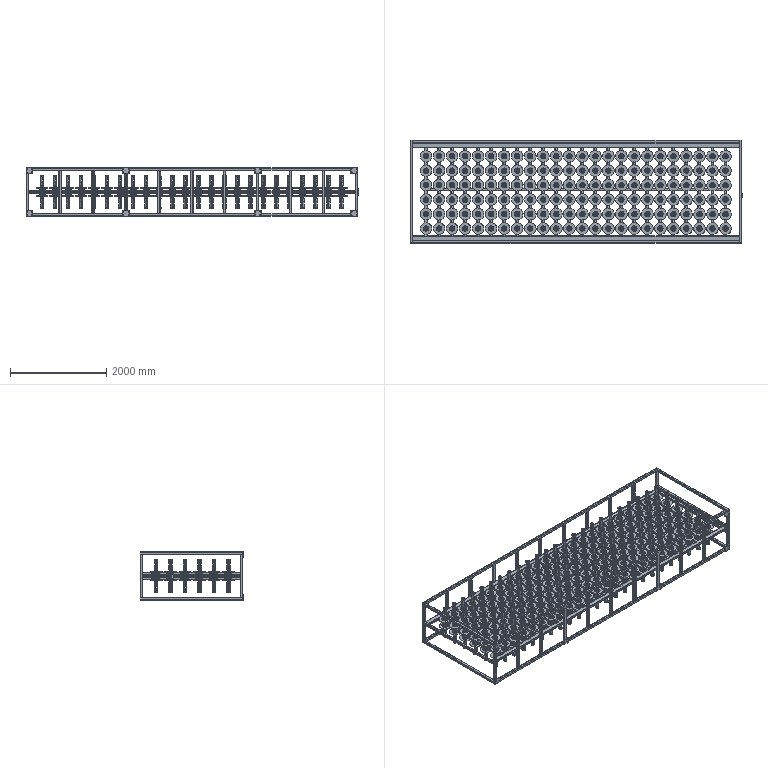Part | SolidWorks | features ReferencePattern 238, LocalLPattern 4, MirrorCompFeat 2, LayoutProfileFeature 1 | 1207 solids | 90272 faces | volume 274546419 mm3 | cylinder 37918 | torus 20736 | plane 17934 | cone 12532 | spline 1152 | commonest cylinder face diameters 60.4 x13248 1 x8064 4.2 x1728 15 x1440 14.3 x1152 42.38 x1152